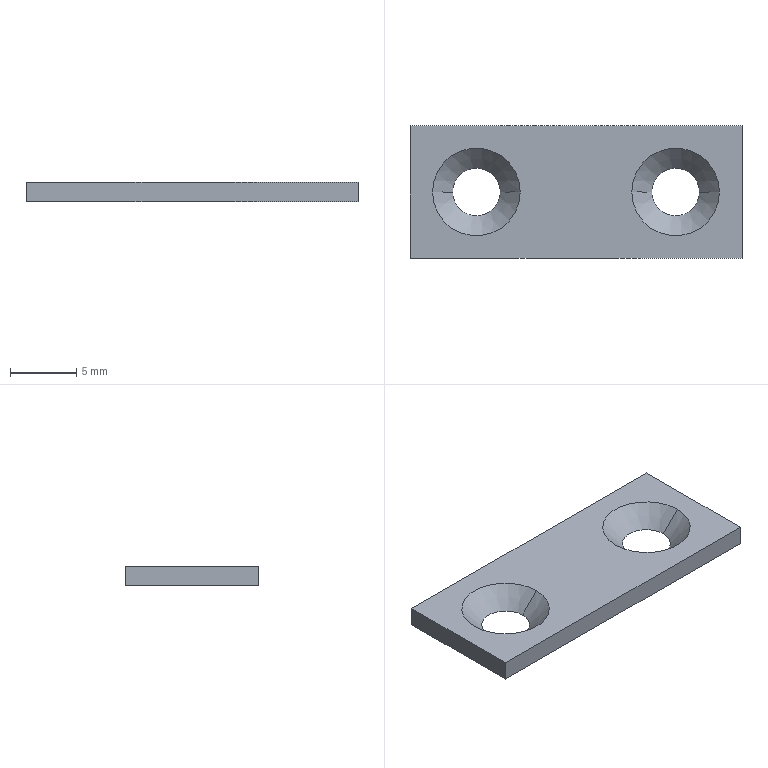Part | STEP file | FBDS-BJ-024 | 1 solid | 10 faces | box 25 x 10 x 1.5 mm | volume 311.948 mm3 | plane 6 | cone 4
STEP:
#1=CARTESIAN_POINT('',(-9.3,0.,-1.5));
#2=VERTEX_POINT('',#1);
#3=CARTESIAN_POINT('',(-5.7,0.,-1.5));
#4=VERTEX_POINT('',#3);
#5=CARTESIAN_POINT('',(-7.5,0.,-1.5));
#6=DIRECTION('',(0.,0.,1.));
#7=DIRECTION('',(1.,0.,0.));
#8=AXIS2_PLACEMENT_3D('',#5,#6,#7);
#9=CIRCLE('',#8,1.8);
#10=EDGE_CURVE('',#2,#4,#9,.T.);
#11=ORIENTED_EDGE('',*,*,#10,.F.);
#12=CARTESIAN_POINT('',(-10.8,0.,0.));
#13=VERTEX_POINT('',#12);
#14=CARTESIAN_POINT('',(-10.8,0.,0.));
#15=DIRECTION('',(-0.7071,0.,0.7071));
#16=VECTOR('',#15,1000.);
#17=LINE('',#14,#16);
#18=EDGE_CURVE('',#2,#13,#17,.T.);
#19=ORIENTED_EDGE('',*,*,#18,.T.);
#20=CARTESIAN_POINT('',(-4.2,0.,0.));
#21=VERTEX_POINT('',#20);
#22=CARTESIAN_POINT('',(-7.5,0.,0.));
#23=DIRECTION('',(0.,0.,1.));
#24=DIRECTION('',(1.,0.,0.));
#25=AXIS2_PLACEMENT_3D('',#22,#23,#24);
#26=CIRCLE('',#25,3.3);
#27=EDGE_CURVE('',#13,#21,#26,.T.);
#28=ORIENTED_EDGE('',*,*,#27,.T.);
#29=CARTESIAN_POINT('',(-4.2,0.,0.));
#30=DIRECTION('',(0.7071,0.,0.7071));
#31=VECTOR('',#30,1000.);
#32=LINE('',#29,#31);
#33=EDGE_CURVE('',#4,#21,#32,.T.);
#34=ORIENTED_EDGE('',*,*,#33,.F.);
#35=EDGE_LOOP('',(#11,#19,#28,#34));
#36=FACE_OUTER_BOUND('',#35,.T.);
#37=CARTESIAN_POINT('',(-7.5,0.,0.));
#38=DIRECTION('',(0.,0.,1.));
#39=DIRECTION('',(1.,0.,0.));
#40=AXIS2_PLACEMENT_3D('',#37,#38,#39);
#41=CONICAL_SURFACE('',#40,3.3,0.7854);
#42=ADVANCED_FACE('',(#36),#41,.F.);
#43=CARTESIAN_POINT('',(5.7,0.,-1.5));
#44=VERTEX_POINT('',#43);
#45=CARTESIAN_POINT('',(9.3,0.,-1.5));
#46=VERTEX_POINT('',#45);
#47=CARTESIAN_POINT('',(7.5,0.,-1.5));
#48=DIRECTION('',(0.,0.,1.));
#49=DIRECTION('',(1.,0.,0.));
#50=AXIS2_PLACEMENT_3D('',#47,#48,#49);
#51=CIRCLE('',#50,1.8);
#52=EDGE_CURVE('',#44,#46,#51,.T.);
#53=ORIENTED_EDGE('',*,*,#52,.F.);
#54=CARTESIAN_POINT('',(4.2,0.,0.));
#55=VERTEX_POINT('',#54);
#56=CARTESIAN_POINT('',(4.2,0.,0.));
#57=DIRECTION('',(-0.7071,0.,0.7071));
#58=VECTOR('',#57,1000.);
#59=LINE('',#56,#58);
#60=EDGE_CURVE('',#44,#55,#59,.T.);
#61=ORIENTED_EDGE('',*,*,#60,.T.);
#62=CARTESIAN_POINT('',(10.8,0.,0.));
#63=VERTEX_POINT('',#62);
#64=CARTESIAN_POINT('',(7.5,0.,0.));
#65=DIRECTION('',(0.,0.,1.));
#66=DIRECTION('',(1.,0.,0.));
#67=AXIS2_PLACEMENT_3D('',#64,#65,#66);
#68=CIRCLE('',#67,3.3);
#69=EDGE_CURVE('',#55,#63,#68,.T.);
#70=ORIENTED_EDGE('',*,*,#69,.T.);
#71=CARTESIAN_POINT('',(10.8,0.,0.));
#72=DIRECTION('',(0.7071,0.,0.7071));
#73=VECTOR('',#72,1000.);
#74=LINE('',#71,#73);
#75=EDGE_CURVE('',#46,#63,#74,.T.);
#76=ORIENTED_EDGE('',*,*,#75,.F.);
#77=EDGE_LOOP('',(#53,#61,#70,#76));
#78=FACE_OUTER_BOUND('',#77,.T.);
#79=CARTESIAN_POINT('',(7.5,0.,0.));
#80=DIRECTION('',(0.,0.,1.));
#81=DIRECTION('',(1.,0.,0.));
#82=AXIS2_PLACEMENT_3D('',#79,#80,#81);
#83=CONICAL_SURFACE('',#82,3.3,0.7854);
#84=ADVANCED_FACE('',(#78),#83,.F.);
#85=CARTESIAN_POINT('',(12.5,-5.,0.));
#86=VERTEX_POINT('',#85);
#87=CARTESIAN_POINT('',(12.5,5.,0.));
#88=VERTEX_POINT('',#87);
#89=CARTESIAN_POINT('',(12.5,5.,0.));
#90=DIRECTION('',(0.,1.,0.));
#91=VECTOR('',#90,1000.);
#92=LINE('',#89,#91);
#93=EDGE_CURVE('',#86,#88,#92,.T.);
#94=ORIENTED_EDGE('',*,*,#93,.F.);
#95=CARTESIAN_POINT('',(12.5,-5.,-1.5));
#96=VERTEX_POINT('',#95);
#97=CARTESIAN_POINT('',(12.5,-5.,-1.5));
#98=DIRECTION('',(0.,0.,1.));
#99=VECTOR('',#98,1000.);
#100=LINE('',#97,#99);
#101=EDGE_CURVE('',#96,#86,#100,.T.);
#102=ORIENTED_EDGE('',*,*,#101,.F.);
#103=CARTESIAN_POINT('',(12.5,5.,-1.5));
#104=VERTEX_POINT('',#103);
#105=CARTESIAN_POINT('',(12.5,5.,-1.5));
#106=DIRECTION('',(0.,1.,0.));
#107=VECTOR('',#106,1000.);
#108=LINE('',#105,#107);
#109=EDGE_CURVE('',#96,#104,#108,.T.);
#110=ORIENTED_EDGE('',*,*,#109,.T.);
#111=CARTESIAN_POINT('',(12.5,5.,-1.5));
#112=DIRECTION('',(0.,0.,1.));
#113=VECTOR('',#112,1000.);
#114=LINE('',#111,#113);
#115=EDGE_CURVE('',#104,#88,#114,.T.);
#116=ORIENTED_EDGE('',*,*,#115,.T.);
#117=EDGE_LOOP('',(#94,#102,#110,#116));
#118=FACE_OUTER_BOUND('',#117,.T.);
#119=CARTESIAN_POINT('',(12.5,5.,-1.5));
#120=DIRECTION('',(1.,0.,0.));
#121=DIRECTION('',(0.,0.,-1.));
#122=AXIS2_PLACEMENT_3D('',#119,#120,#121);
#123=PLANE('',#122);
#124=ADVANCED_FACE('',(#118),#123,.T.);
#125=CARTESIAN_POINT('',(-12.5,-5.,0.));
#126=VERTEX_POINT('',#125);
#127=CARTESIAN_POINT('',(-12.5,-5.,0.));
#128=DIRECTION('',(1.,0.,0.));
#129=VECTOR('',#128,1000.);
#130=LINE('',#127,#129);
#131=EDGE_CURVE('',#126,#86,#130,.T.);
#132=ORIENTED_EDGE('',*,*,#131,.F.);
#133=CARTESIAN_POINT('',(-12.5,-5.,-1.5));
#134=VERTEX_POINT('',#133);
#135=CARTESIAN_POINT('',(-12.5,-5.,-1.5));
#136=DIRECTION('',(0.,0.,1.));
#137=VECTOR('',#136,1000.);
#138=LINE('',#135,#137);
#139=EDGE_CURVE('',#134,#126,#138,.T.);
#140=ORIENTED_EDGE('',*,*,#139,.F.);
#141=CARTESIAN_POINT('',(-12.5,-5.,-1.5));
#142=DIRECTION('',(1.,0.,0.));
#143=VECTOR('',#142,1000.);
#144=LINE('',#141,#143);
#145=EDGE_CURVE('',#134,#96,#144,.T.);
#146=ORIENTED_EDGE('',*,*,#145,.T.);
#147=ORIENTED_EDGE('',*,*,#101,.T.);
#148=EDGE_LOOP('',(#132,#140,#146,#147));
#149=FACE_OUTER_BOUND('',#148,.T.);
#150=CARTESIAN_POINT('',(-12.5,-5.,-1.5));
#151=DIRECTION('',(0.,-1.,0.));
#152=DIRECTION('',(0.,0.,-1.));
#153=AXIS2_PLACEMENT_3D('',#150,#151,#152);
#154=PLANE('',#153);
#155=ADVANCED_FACE('',(#149),#154,.T.);
#156=CARTESIAN_POINT('',(-12.5,5.,0.));
#157=VERTEX_POINT('',#156);
#158=CARTESIAN_POINT('',(-12.5,5.,0.));
#159=DIRECTION('',(0.,-1.,0.));
#160=VECTOR('',#159,1000.);
#161=LINE('',#158,#160);
#162=EDGE_CURVE('',#157,#126,#161,.T.);
#163=ORIENTED_EDGE('',*,*,#162,.F.);
#164=CARTESIAN_POINT('',(-12.5,5.,-1.5));
#165=VERTEX_POINT('',#164);
#166=CARTESIAN_POINT('',(-12.5,5.,-1.5));
#167=DIRECTION('',(0.,0.,1.));
#168=VECTOR('',#167,1000.);
#169=LINE('',#166,#168);
#170=EDGE_CURVE('',#165,#157,#169,.T.);
#171=ORIENTED_EDGE('',*,*,#170,.F.);
#172=CARTESIAN_POINT('',(-12.5,5.,-1.5));
#173=DIRECTION('',(0.,-1.,0.));
#174=VECTOR('',#173,1000.);
#175=LINE('',#172,#174);
#176=EDGE_CURVE('',#165,#134,#175,.T.);
#177=ORIENTED_EDGE('',*,*,#176,.T.);
#178=ORIENTED_EDGE('',*,*,#139,.T.);
#179=EDGE_LOOP('',(#163,#171,#177,#178));
#180=FACE_OUTER_BOUND('',#179,.T.);
#181=CARTESIAN_POINT('',(-12.5,5.,-1.5));
#182=DIRECTION('',(-1.,0.,0.));
#183=DIRECTION('',(0.,-1.,0.));
#184=AXIS2_PLACEMENT_3D('',#181,#182,#183);
#185=PLANE('',#184);
#186=ADVANCED_FACE('',(#180),#185,.T.);
#187=CARTESIAN_POINT('',(-12.5,5.,0.));
#188=DIRECTION('',(-1.,0.,0.));
#189=VECTOR('',#188,1000.);
#190=LINE('',#187,#189);
#191=EDGE_CURVE('',#88,#157,#190,.T.);
#192=ORIENTED_EDGE('',*,*,#191,.F.);
#193=ORIENTED_EDGE('',*,*,#115,.F.);
#194=CARTESIAN_POINT('',(-12.5,5.,-1.5));
#195=DIRECTION('',(-1.,0.,0.));
#196=VECTOR('',#195,1000.);
#197=LINE('',#194,#196);
#198=EDGE_CURVE('',#104,#165,#197,.T.);
#199=ORIENTED_EDGE('',*,*,#198,.T.);
#200=ORIENTED_EDGE('',*,*,#170,.T.);
#201=EDGE_LOOP('',(#192,#193,#199,#200));
#202=FACE_OUTER_BOUND('',#201,.T.);
#203=CARTESIAN_POINT('',(-12.5,5.,-1.5));
#204=DIRECTION('',(0.,1.,0.));
#205=DIRECTION('',(0.,0.,1.));
#206=AXIS2_PLACEMENT_3D('',#203,#204,#205);
#207=PLANE('',#206);
#208=ADVANCED_FACE('',(#202),#207,.T.);
#209=CARTESIAN_POINT('',(-7.5,0.,-1.5));
#210=DIRECTION('',(0.,0.,1.));
#211=DIRECTION('',(1.,0.,0.));
#212=AXIS2_PLACEMENT_3D('',#209,#210,#211);
#213=CIRCLE('',#212,1.8);
#214=EDGE_CURVE('',#4,#2,#213,.T.);
#215=ORIENTED_EDGE('',*,*,#214,.T.);
#216=ORIENTED_EDGE('',*,*,#10,.T.);
#217=EDGE_LOOP('',(#215,#216));
#218=FACE_BOUND('',#217,.T.);
#219=CARTESIAN_POINT('',(7.5,0.,-1.5));
#220=DIRECTION('',(0.,0.,1.));
#221=DIRECTION('',(1.,0.,0.));
#222=AXIS2_PLACEMENT_3D('',#219,#220,#221);
#223=CIRCLE('',#222,1.8);
#224=EDGE_CURVE('',#46,#44,#223,.T.);
#225=ORIENTED_EDGE('',*,*,#224,.T.);
#226=ORIENTED_EDGE('',*,*,#52,.T.);
#227=EDGE_LOOP('',(#225,#226));
#228=FACE_BOUND('',#227,.T.);
#229=ORIENTED_EDGE('',*,*,#109,.F.);
#230=ORIENTED_EDGE('',*,*,#145,.F.);
#231=ORIENTED_EDGE('',*,*,#176,.F.);
#232=ORIENTED_EDGE('',*,*,#198,.F.);
#233=EDGE_LOOP('',(#229,#230,#231,#232));
#234=FACE_OUTER_BOUND('',#233,.T.);
#235=CARTESIAN_POINT('',(0.,0.,-1.5));
#236=DIRECTION('',(0.,0.,1.));
#237=DIRECTION('',(1.,0.,0.));
#238=AXIS2_PLACEMENT_3D('',#235,#236,#237);
#239=PLANE('',#238);
#240=ADVANCED_FACE('',(#218,#228,#234),#239,.F.);
#241=CARTESIAN_POINT('',(-7.5,0.,0.));
#242=DIRECTION('',(0.,0.,1.));
#243=DIRECTION('',(1.,0.,0.));
#244=AXIS2_PLACEMENT_3D('',#241,#242,#243);
#245=CIRCLE('',#244,3.3);
#246=EDGE_CURVE('',#21,#13,#245,.T.);
#247=ORIENTED_EDGE('',*,*,#246,.F.);
#248=ORIENTED_EDGE('',*,*,#27,.F.);
#249=EDGE_LOOP('',(#247,#248));
#250=FACE_BOUND('',#249,.T.);
#251=CARTESIAN_POINT('',(7.5,0.,0.));
#252=DIRECTION('',(0.,0.,1.));
#253=DIRECTION('',(1.,0.,0.));
#254=AXIS2_PLACEMENT_3D('',#251,#252,#253);
#255=CIRCLE('',#254,3.3);
#256=EDGE_CURVE('',#63,#55,#255,.T.);
#257=ORIENTED_EDGE('',*,*,#256,.F.);
#258=ORIENTED_EDGE('',*,*,#69,.F.);
#259=EDGE_LOOP('',(#257,#258));
#260=FACE_BOUND('',#259,.T.);
#261=ORIENTED_EDGE('',*,*,#93,.T.);
#262=ORIENTED_EDGE('',*,*,#191,.T.);
#263=ORIENTED_EDGE('',*,*,#162,.T.);
#264=ORIENTED_EDGE('',*,*,#131,.T.);
#265=EDGE_LOOP('',(#261,#262,#263,#264));
#266=FACE_OUTER_BOUND('',#265,.T.);
#267=CARTESIAN_POINT('',(0.,0.,0.));
#268=DIRECTION('',(0.,0.,1.));
#269=DIRECTION('',(1.,0.,0.));
#270=AXIS2_PLACEMENT_3D('',#267,#268,#269);
#271=PLANE('',#270);
#272=ADVANCED_FACE('',(#250,#260,#266),#271,.T.);
#273=ORIENTED_EDGE('',*,*,#60,.F.);
#274=ORIENTED_EDGE('',*,*,#224,.F.);
#275=ORIENTED_EDGE('',*,*,#75,.T.);
#276=ORIENTED_EDGE('',*,*,#256,.T.);
#277=EDGE_LOOP('',(#273,#274,#275,#276));
#278=FACE_OUTER_BOUND('',#277,.T.);
#279=CARTESIAN_POINT('',(7.5,0.,0.));
#280=DIRECTION('',(0.,0.,1.));
#281=DIRECTION('',(1.,0.,0.));
#282=AXIS2_PLACEMENT_3D('',#279,#280,#281);
#283=CONICAL_SURFACE('',#282,3.3,0.7854);
#284=ADVANCED_FACE('',(#278),#283,.F.);
#285=ORIENTED_EDGE('',*,*,#18,.F.);
#286=ORIENTED_EDGE('',*,*,#214,.F.);
#287=ORIENTED_EDGE('',*,*,#33,.T.);
#288=ORIENTED_EDGE('',*,*,#246,.T.);
#289=EDGE_LOOP('',(#285,#286,#287,#288));
#290=FACE_OUTER_BOUND('',#289,.T.);
#291=CARTESIAN_POINT('',(-7.5,0.,0.));
#292=DIRECTION('',(0.,0.,1.));
#293=DIRECTION('',(1.,0.,0.));
#294=AXIS2_PLACEMENT_3D('',#291,#292,#293);
#295=CONICAL_SURFACE('',#294,3.3,0.7854);
#296=ADVANCED_FACE('',(#290),#295,.F.);
#297=CLOSED_SHELL('',(#42,#84,#124,#155,#186,#208,#240,#272,#284,#296));
#298=MANIFOLD_SOLID_BREP('',#297);
#299=CARTESIAN_POINT('',(0.,0.,0.));
#300=DIRECTION('',(0.,0.,1.));
#301=DIRECTION('',(1.,0.,0.));
#302=AXIS2_PLACEMENT_3D('',#299,#300,#301);
#303=(LENGTH_UNIT()NAMED_UNIT(*)SI_UNIT(.MILLI.,.METRE.));
#304=UNCERTAINTY_MEASURE_WITH_UNIT(LENGTH_MEASURE(0.00001),#303,'','');
#305=(NAMED_UNIT(*)PLANE_ANGLE_UNIT()SI_UNIT($,.RADIAN.));
#306=(NAMED_UNIT(*)SI_UNIT($,.STERADIAN.)SOLID_ANGLE_UNIT());
#307=(GEOMETRIC_REPRESENTATION_CONTEXT(3)GLOBAL_UNCERTAINTY_ASSIGNED_CONTEXT((#304))GLOBAL_UNIT_ASSIGNED_CONTEXT((#303,#305,#306))REPRESENTATION_CONTEXT('',''));
#308=ADVANCED_BREP_SHAPE_REPRESENTATION('',(#298,#302),#307);